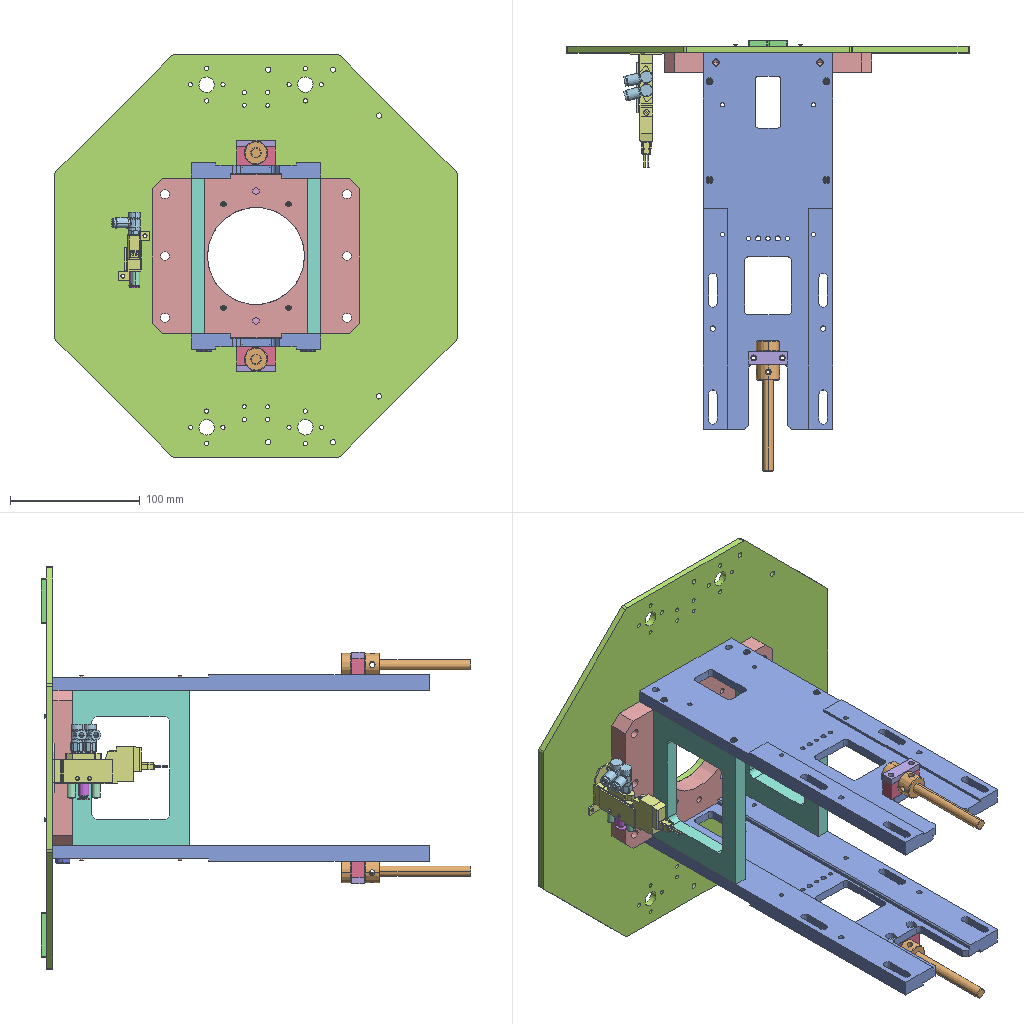Assembly | SolidWorks | 15 different items | 42 placed | box 310 x 331 x 310 mm
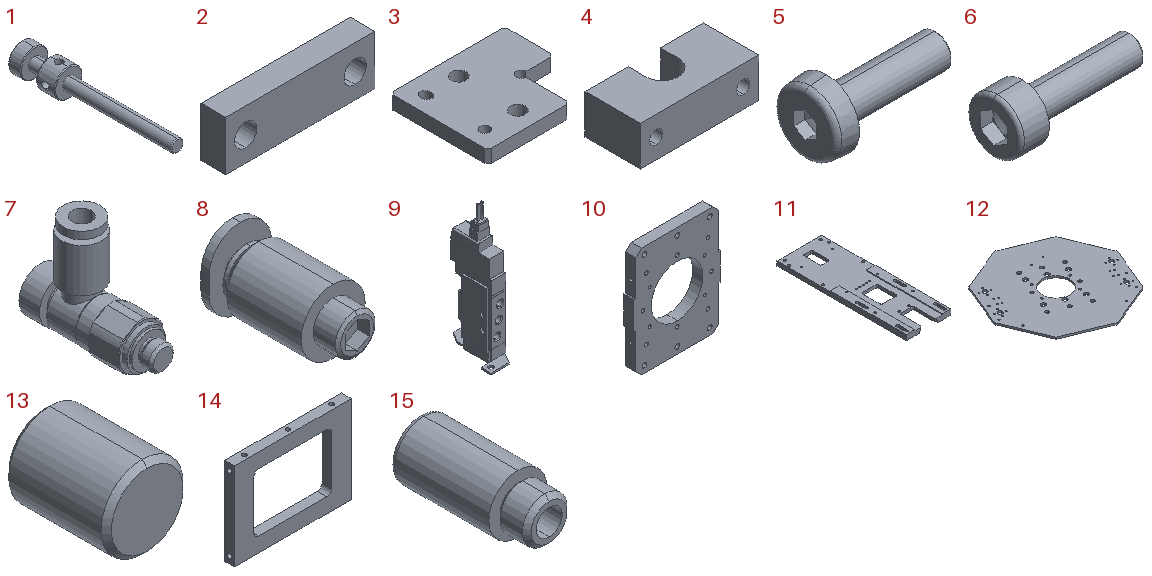Parts list (item | quantity | size | volume | features):
1 | x2 | 18 x 100 x 18 mm | 8573 mm3 | features ICE 4, Chamfer 2, CirPattern 1, Extrusion 1
2 | x2 | 30 x 5 x 10 mm | 1341 mm3 | features Extrusion 1, ICE 1
3 | x2 | 35 x 30 x 4 mm | 3379 mm3 | features HoleWzd 3, ICE 2, Chamfer 1, Extrusion 1
4 | x2 | 30 x 14 x 10 mm | 3327 mm3 | features Extrusion 1, HoleWzd 1, ICE 1
5 | x2 | 23.9 x 12 x 12 mm | 939.348 mm3 | features Cut 2, Fillet 2, Boss 1, Chamfer 1, Extrusion 1, LPattern 1, RevCut 1
6 | x18 | 7.6 x 3 x 3 mm | 21.652 mm3 | features Fillet 2, RevCut 2, Boss 1, Chamfer 1, Cut 1, Extrusion 1, LPattern 1
7 | x2 | 9.373 x 25.4 x 22 mm | 1869 mm3 | features Revolution 2, ICE 1, RevCut 1
8 | x1 | 8 x 15.6 x 9.8 mm | 520.13 mm3 | features BaseBody 1
9 | x1 | 24.041 x 38 x 88.25 mm | 16472 mm3 | features BaseBody 1
10 | x1 | 126 x 15 x 160 mm | 213891 mm3 | features Cut 5, ICE 4, 3DProfileFeature 3, HoleWzd 3, Chamfer 2, Extrusion 1, MirrorPattern 1
11 | x2 | 100 x 290 x 12 mm | 225804 mm3 | features ICE 9, HoleWzd 5, Chamfer 2, LPattern 2, 3DProfileFeature 1, Extrusion 1, Fillet 1
12 | x1 | 335.047 x 335.047 x 5 mm | 365472 mm3 | features HoleWzd 5, ICE 5, Cut 4, 3DProfileFeature 2, Extrusion 1, Fillet 1
13 | x2 | 8 x 10 x 8 mm | 496.633 mm3 | features Chamfer 1, Extrusion 1
14 | x2 | 120 x 10 x 90 mm | 58973 mm3 | features 3DProfileFeature 2, Cut 2, HoleWzd 2, Extrusion 1, ICE 1, MirrorPattern 1
15 | x2 | 6.5 x 15 x 6.5 mm | 404.686 mm3 | features BaseBody 1
Mates (type | each side: item.copy, entity, surface, feature):
Coincident | 11.1 face plane Boss-Extrude1 | 10.1 face plane Boss-Extrude1
Coincident | 10.1 face plane Boss-Extrude1 | 11.2 face plane Boss-Extrude1 | 2 times
Coincident | 10.1 face plane Boss-Extrude1 | 11.1 face plane Boss-Extrude1 | 2 times
Coincident | 11.1 face plane Boss-Extrude1 | 11.2 face plane Boss-Extrude1
Coincident | 10.1 face plane Boss-Extrude1 | 12.1 face plane Boss-Extrude1
Concentric | 10.1 face cylinder Cut-Extrude1 | 12.1 face cylinder Cut-Extrude1
Parallel | 10.1 face plane Boss-Extrude1 | 12.1 face plane Boss-Extrude1
Concentric | 12.1 face cylinder Cut-Extrude3 | 6.1 face cylinder BaseBody
Coincident | 12.1 face plane Boss-Extrude1 | 6.1 face plane BaseHead
Concentric | 12.1 face cylinder Cut-Extrude3 | 6.2 face cylinder BaseBody
Coincident | 12.1 face plane Boss-Extrude1 | 6.2 face plane BaseHead
Concentric | 12.1 face cylinder Cut-Extrude3 | 6.3 face cylinder BaseBody
Coincident | 12.1 face plane Boss-Extrude1 | 6.3 face plane BaseHead
Concentric | 12.1 face cylinder Cut-Extrude3 | 6.4 face cylinder BaseBody
Coincident | 12.1 face plane Boss-Extrude1 | 6.4 face plane BaseHead
Coincident | 10.1 face plane Cut-Extrude6 | 13.1 face plane Boss-Extrude1
Concentric | 10.1 face cylinder Cut-Extrude6 | 13.1 face cylinder Boss-Extrude1
Coincident | 10.1 face plane Cut-Extrude6 | 13.2 face plane Boss-Extrude1
Concentric | 10.1 face cylinder Cut-Extrude6 | 13.2 face cylinder Boss-Extrude1
Coincident | 11.2 face plane Boss-Extrude1 | 14.1 face plane Boss-Extrude1
Coincident | 11.1 face plane Boss-Extrude1 | 14.1 face plane Boss-Extrude1
Coincident | 10.1 face plane Boss-Extrude1 | 14.1 face plane Boss-Extrude1
Concentric | 11.1 face cylinder LPattern1 | 6.5 face cylinder BaseBody
Coincident | 11.1 face plane Boss-Extrude1 | 6.5 face plane BaseHead
Concentric | 11.1 face cylinder Cut-Extrude4 | 6.6 face cylinder BaseBody
Coincident | 11.1 face plane Boss-Extrude1 | 6.6 face plane BaseHead
Concentric | 11.1 face cylinder Cut-Extrude4 | 6.7 face cylinder BaseBody
Coincident | 11.1 face plane Boss-Extrude1 | 6.7 face plane BaseHead
Concentric | 11.1 face cylinder LPattern1 | 6.8 face cylinder BaseBody
Coincident | 11.1 face plane Boss-Extrude1 | 6.8 face plane BaseHead
Concentric | 11.2 face cylinder LPattern1 | 6.9 face cylinder BaseBody
Coincident | 11.2 face plane Boss-Extrude1 | 6.9 face plane BaseHead
Concentric | 11.2 face cylinder Cut-Extrude4 | 6.10 face cylinder BaseBody
Coincident | 11.2 face plane Boss-Extrude1 | 6.10 face plane BaseHead
Concentric | 11.2 face cylinder Cut-Extrude4 | 6.11 face cylinder BaseBody
Coincident | 11.2 face plane Boss-Extrude1 | 6.11 face plane BaseHead
Concentric | 11.2 face cylinder LPattern1 | 6.12 face cylinder BaseBody
Coincident | 11.2 face plane Boss-Extrude1 | 6.12 face plane BaseHead
Coincident | 10.1 face plane Boss-Extrude2 | 11.1 face plane Cut-Extrude3
Concentric | 11.2 face cylinder Cut-Extrude8 | 5.1 face cylinder BaseBody
Coincident | 11.2 face plane Boss-Extrude1 | 5.1 face plane BaseHead
Concentric | 11.2 face cylinder Cut-Extrude8 | 5.2 face cylinder BaseBody
Coincident | 11.2 face plane Boss-Extrude1 | 5.2 face plane BaseHead
Coincident | 10.1 face plane Boss-Extrude1 | 14.2 face plane Boss-Extrude1
Coincident | 11.1 face plane Boss-Extrude1 | 14.2 face plane Boss-Extrude1
Coincident | 11.2 face plane Boss-Extrude1 | 14.2 face plane Boss-Extrude1
Concentric | 10.1 face cylinder Cut-Extrude8 | 6.13 face cylinder BaseBody
Coincident | 10.1 face plane Cut-Extrude9 | 6.13 face plane BaseHead
Concentric | 10.1 face cylinder Cut-Extrude8 | 6.14 face cylinder BaseBody
Coincident | 10.1 face plane Cut-Extrude9 | 6.14 face plane BaseHead
Concentric | 10.1 face cylinder Cut-Extrude8 | 6.15 face cylinder BaseBody
Coincident | 10.1 face plane Cut-Extrude9 | 6.15 face plane BaseHead
Concentric | 10.1 face cylinder Cut-Extrude8 | 6.16 face cylinder BaseBody
Coincident | 10.1 face plane Cut-Extrude9 | 6.16 face plane BaseHead
Concentric | 10.1 face cylinder Cut-Extrude8 | 6.17 face cylinder BaseBody
Coincident | 10.1 face plane Cut-Extrude9 | 6.17 face plane BaseHead
Concentric | 10.1 face cylinder Cut-Extrude8 | 6.18 face cylinder BaseBody
Coincident | 10.1 face plane Cut-Extrude9 | 6.18 face plane BaseHead
Concentric | 12.1 face cylinder M4 Tapped Hole2 | 3.1 face cylinder Ø4.5 (4.5) Diameter Hole1 | 2 times
Concentric | 12.1 face cylinder M4 Tapped Hole2 | 3.2 face cylinder Ø4.5 (4.5) Diameter Hole1 | 2 times
Coincident | 12.1 face plane Boss-Extrude1 | 3.2 face plane Boss-Extrude1
Coincident | 12.1 face plane Boss-Extrude1 | 3.1 face plane Boss-Extrude1
Coincident | 12.1 face plane Boss-Extrude1 | 9.1 face plane Input1
Width | 9.1 face plane Input1 | 9.1 face plane Input1 | 10.1 face plane Boss-Extrude1 | 10.1 face plane Boss-Extrude1
Coincident | 9.1 face plane Input1 | 15.1 face plane Input1
Coincident | 9.1 face plane Input1 | 15.2 face plane Input1
Concentric | 9.1 face cylinder Input1 | 15.1 face cylinder Input1
Concentric | 9.1 face cylinder Input1 | 15.2 face cylinder Input1
Concentric | 9.1 face cylinder Input1 | 8.1 face cylinder Input1
Coincident | 9.1 face plane Input1 | 8.1 face plane Input1
DistanceDim | 9.1 face plane Input1 | 10.1 face plane Boss-Extrude1
Concentric | 4.1 face cylinder M4 Tapped Hole1 | 11.2 face cylinder Hole size per socket head cap screw type1
Concentric | 11.2 face cylinder Hole size per socket head cap screw type1 | 4.1 face cylinder M4 Tapped Hole1
Coincident | 11.2 face plane Boss-Extrude1 | 4.1 face plane Boss-Extrude1
Concentric | 2.1 face cylinder Cut-Extrude1 | 4.1 face cylinder M4 Tapped Hole1 | 2 times
Coincident | 2.1 face plane Boss-Extrude1 | 4.1 face plane Boss-Extrude1
Coincident | 1.1 face plane Boss-Extrude2 | 4.1 face plane Boss-Extrude1
Concentric | 1.1 face cylinder Boss-Extrude1 | 4.1 face cylinder Cut-Extrude1
Concentric | 11.1 face cylinder Hole size per socket head cap screw type1 | 4.2 face cylinder M4 Tapped Hole1 | 2 times
Coincident | 11.1 face plane Boss-Extrude1 | 4.2 face plane Boss-Extrude1
Concentric | 2.2 face cylinder Cut-Extrude1 | 4.2 face cylinder M4 Tapped Hole1 | 2 times
Coincident | 2.2 face plane Boss-Extrude1 | 4.2 face plane Boss-Extrude1
Coincident | 1.2 face plane Boss-Extrude2 | 4.2 face plane Boss-Extrude1
Concentric | 1.2 face cylinder Boss-Extrude1 | 4.2 face cylinder Cut-Extrude1
Coincident | 9.1 edge | 7.1 face plane Revolve1
Concentric | 9.1 face cylinder Input1 | 7.1 face cylinder Revolve1
Coincident | 9.1 edge | 7.2 face plane Revolve1
Concentric | 9.1 face cylinder Input1 | 7.2 face cylinder Revolve1